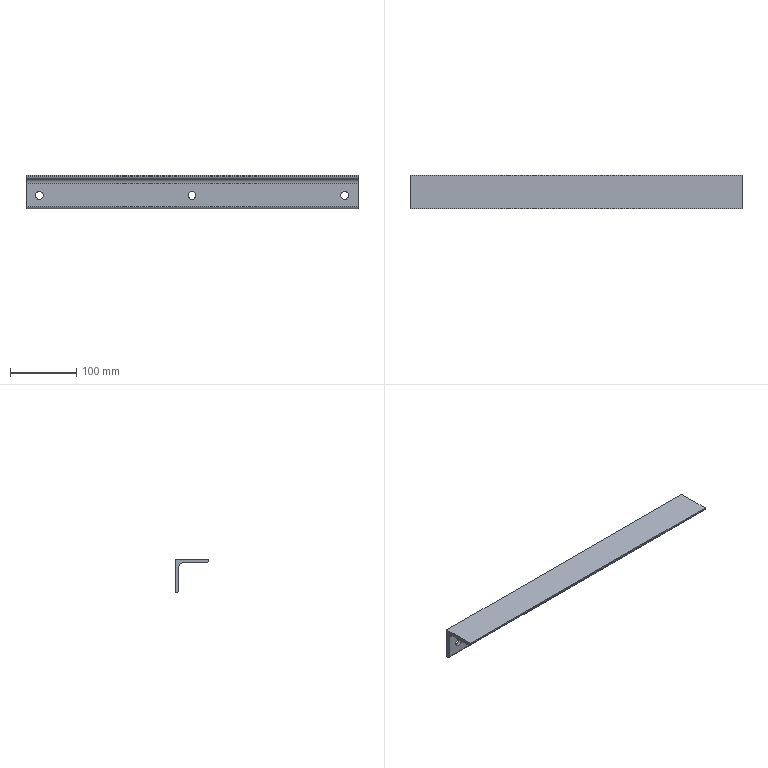Part | STEP file | Input 114 | 1 solid | 17 faces | box 500 x 50 x 50 mm | volume 238406 mm3 | cylinder 9 | plane 8 | commonest cylinder face diameters 12 x6 6 x2 13 x1
STEP:
#1=CARTESIAN_POINT('',(0.,0.,0.));
#2=DIRECTION('',(0.,0.,1.));
#3=DIRECTION('',(1.,0.,0.));
#4=AXIS2_PLACEMENT_3D('',#1,#2,#3);
#5=CARTESIAN_POINT('',(2524.,319.5,-230.));
#6=VERTEX_POINT('',#5);
#7=CARTESIAN_POINT('',(2524.,324.5,-230.));
#8=VERTEX_POINT('',#7);
#9=CARTESIAN_POINT('',(2524.,239.499,-230.));
#10=DIRECTION('',(0.,1.,0.));
#11=VECTOR('',#10,1.);
#12=LINE('',#9,#11);
#13=CARTESIAN_POINT('',(2530.,239.499,-230.));
#14=DIRECTION('',(0.,1.,0.));
#15=DIRECTION('',(-1.,0.,0.));
#16=AXIS2_PLACEMENT_3D('',#13,#14,#15);
#17=CYLINDRICAL_SURFACE('',#16,6.);
#18=CARTESIAN_POINT('',(6.283,0.));
#19=DIRECTION('',(0.,1.));
#20=VECTOR('',#19,1.);
#21=LINE('',#18,#20);
#22=(GEOMETRIC_REPRESENTATION_CONTEXT(2)PARAMETRIC_REPRESENTATION_CONTEXT()REPRESENTATION_CONTEXT('',''));
#23=DEFINITIONAL_REPRESENTATION('',(#21),#22);
#24=PCURVE('',#17,#23);
#25=CARTESIAN_POINT('',(2530.,239.499,-230.));
#26=DIRECTION('',(0.,1.,0.));
#27=DIRECTION('',(-1.,0.,0.));
#28=AXIS2_PLACEMENT_3D('',#25,#26,#27);
#29=CYLINDRICAL_SURFACE('',#28,6.);
#30=CARTESIAN_POINT('',(0.,0.));
#31=DIRECTION('',(0.,1.));
#32=VECTOR('',#31,1.);
#33=LINE('',#30,#32);
#34=(GEOMETRIC_REPRESENTATION_CONTEXT(2)PARAMETRIC_REPRESENTATION_CONTEXT()REPRESENTATION_CONTEXT('',''));
#35=DEFINITIONAL_REPRESENTATION('',(#33),#34);
#36=PCURVE('',#29,#35);
#37=SURFACE_CURVE('',#12,(#24,#36),.PCURVE_S1.);
#38=EDGE_CURVE('',#6,#8,#37,.T.);
#39=ORIENTED_EDGE('',*,*,#38,.T.);
#40=CARTESIAN_POINT('',(2536.,324.5,-230.));
#41=VERTEX_POINT('',#40);
#42=CARTESIAN_POINT('',(2530.,324.5,-230.));
#43=DIRECTION('',(0.,1.,0.));
#44=DIRECTION('',(-1.,0.,0.));
#45=AXIS2_PLACEMENT_3D('',#42,#43,#44);
#46=CIRCLE('',#45,6.);
#47=CARTESIAN_POINT('',(0.,85.001));
#48=DIRECTION('',(1.,0.));
#49=VECTOR('',#48,1.);
#50=LINE('',#47,#49);
#51=(GEOMETRIC_REPRESENTATION_CONTEXT(2)PARAMETRIC_REPRESENTATION_CONTEXT()REPRESENTATION_CONTEXT('',''));
#52=DEFINITIONAL_REPRESENTATION('',(#50),#51);
#53=PCURVE('',#17,#52);
#54=CARTESIAN_POINT('',(2510.,324.5,-200.));
#55=DIRECTION('',(0.,1.,0.));
#56=DIRECTION('',(-1.,0.,0.));
#57=AXIS2_PLACEMENT_3D('',#54,#55,#56);
#58=PLANE('',#57);
#59=CARTESIAN_POINT('',(-20.,-30.));
#60=DIRECTION('',(1.,0.));
#61=AXIS2_PLACEMENT_2D('',#59,#60);
#62=CIRCLE('',#61,6.);
#63=(GEOMETRIC_REPRESENTATION_CONTEXT(2)PARAMETRIC_REPRESENTATION_CONTEXT()REPRESENTATION_CONTEXT('',''));
#64=DEFINITIONAL_REPRESENTATION('',(#62),#63);
#65=PCURVE('',#58,#64);
#66=SURFACE_CURVE('',#46,(#53,#65),.PCURVE_S1.);
#67=EDGE_CURVE('',#41,#8,#66,.T.);
#68=ORIENTED_EDGE('',*,*,#67,.F.);
#69=CARTESIAN_POINT('',(2536.,319.5,-230.));
#70=VERTEX_POINT('',#69);
#71=CARTESIAN_POINT('',(2536.,239.499,-230.));
#72=DIRECTION('',(0.,1.,0.));
#73=VECTOR('',#72,1.);
#74=LINE('',#71,#73);
#75=CARTESIAN_POINT('',(3.142,0.));
#76=DIRECTION('',(0.,1.));
#77=VECTOR('',#76,1.);
#78=LINE('',#75,#77);
#79=(GEOMETRIC_REPRESENTATION_CONTEXT(2)PARAMETRIC_REPRESENTATION_CONTEXT()REPRESENTATION_CONTEXT('',''));
#80=DEFINITIONAL_REPRESENTATION('',(#78),#79);
#81=PCURVE('',#17,#80);
#82=CARTESIAN_POINT('',(3.142,0.));
#83=DIRECTION('',(0.,1.));
#84=VECTOR('',#83,1.);
#85=LINE('',#82,#84);
#86=(GEOMETRIC_REPRESENTATION_CONTEXT(2)PARAMETRIC_REPRESENTATION_CONTEXT()REPRESENTATION_CONTEXT('',''));
#87=DEFINITIONAL_REPRESENTATION('',(#85),#86);
#88=PCURVE('',#29,#87);
#89=SURFACE_CURVE('',#74,(#81,#88),.PCURVE_S1.);
#90=EDGE_CURVE('',#70,#41,#89,.T.);
#91=ORIENTED_EDGE('',*,*,#90,.F.);
#92=CARTESIAN_POINT('',(2530.,319.5,-230.));
#93=DIRECTION('',(0.,1.,0.));
#94=DIRECTION('',(0.,0.,1.));
#95=AXIS2_PLACEMENT_3D('',#92,#93,#94);
#96=CIRCLE('',#95,6.);
#97=CARTESIAN_POINT('',(1.571,80.001));
#98=DIRECTION('',(1.,0.));
#99=VECTOR('',#98,1.);
#100=LINE('',#97,#99);
#101=(GEOMETRIC_REPRESENTATION_CONTEXT(2)PARAMETRIC_REPRESENTATION_CONTEXT()REPRESENTATION_CONTEXT('',''));
#102=DEFINITIONAL_REPRESENTATION('',(#100),#101);
#103=PCURVE('',#17,#102);
#104=CARTESIAN_POINT('',(2510.,319.5,-247.));
#105=DIRECTION('',(0.,-1.,0.));
#106=DIRECTION('',(0.,0.,1.));
#107=AXIS2_PLACEMENT_3D('',#104,#105,#106);
#108=PLANE('',#107);
#109=CARTESIAN_POINT('',(23.,-20.));
#110=CARTESIAN_POINT('',(23.,-30.392));
#111=CARTESIAN_POINT('',(14.,-25.196));
#112=CARTESIAN_POINT('',(5.,-20.));
#113=CARTESIAN_POINT('',(14.,-14.804));
#114=CARTESIAN_POINT('',(23.,-9.608));
#115=CARTESIAN_POINT('',(23.,-20.));
#116=(BOUNDED_CURVE()B_SPLINE_CURVE(2,(#109,#110,#111,#112,#113,#114,#115),.UNSPECIFIED.,.T.,.F.)B_SPLINE_CURVE_WITH_KNOTS((1,2,2,2,2,1),(-2.094,0.,2.094,4.189,6.283,8.378),.UNSPECIFIED.)CURVE()GEOMETRIC_REPRESENTATION_ITEM()RATIONAL_B_SPLINE_CURVE((1.,0.5,1.,0.5,1.,0.5,1.))REPRESENTATION_ITEM(''));
#117=(GEOMETRIC_REPRESENTATION_CONTEXT(2)PARAMETRIC_REPRESENTATION_CONTEXT()REPRESENTATION_CONTEXT('',''));
#118=DEFINITIONAL_REPRESENTATION('',(#116),#117);
#119=PCURVE('',#108,#118);
#120=SURFACE_CURVE('',#96,(#103,#119),.PCURVE_S1.);
#121=EDGE_CURVE('',#70,#6,#120,.T.);
#122=ORIENTED_EDGE('',*,*,#121,.T.);
#123=EDGE_LOOP('',(#39,#68,#91,#122));
#124=FACE_BOUND('',#123,.F.);
#125=ADVANCED_FACE('',(#124),#17,.F.);
#126=CARTESIAN_POINT('',(2754.,319.5,-230.));
#127=VERTEX_POINT('',#126);
#128=CARTESIAN_POINT('',(2754.,324.5,-230.));
#129=VERTEX_POINT('',#128);
#130=CARTESIAN_POINT('',(2754.,239.499,-230.));
#131=DIRECTION('',(0.,1.,0.));
#132=VECTOR('',#131,1.);
#133=LINE('',#130,#132);
#134=CARTESIAN_POINT('',(2760.,239.499,-230.));
#135=DIRECTION('',(0.,1.,0.));
#136=DIRECTION('',(-1.,0.,0.));
#137=AXIS2_PLACEMENT_3D('',#134,#135,#136);
#138=CYLINDRICAL_SURFACE('',#137,6.);
#139=CARTESIAN_POINT('',(6.283,0.));
#140=DIRECTION('',(0.,1.));
#141=VECTOR('',#140,1.);
#142=LINE('',#139,#141);
#143=(GEOMETRIC_REPRESENTATION_CONTEXT(2)PARAMETRIC_REPRESENTATION_CONTEXT()REPRESENTATION_CONTEXT('',''));
#144=DEFINITIONAL_REPRESENTATION('',(#142),#143);
#145=PCURVE('',#138,#144);
#146=CARTESIAN_POINT('',(2760.,239.499,-230.));
#147=DIRECTION('',(0.,1.,0.));
#148=DIRECTION('',(-1.,0.,0.));
#149=AXIS2_PLACEMENT_3D('',#146,#147,#148);
#150=CYLINDRICAL_SURFACE('',#149,6.);
#151=CARTESIAN_POINT('',(0.,0.));
#152=DIRECTION('',(0.,1.));
#153=VECTOR('',#152,1.);
#154=LINE('',#151,#153);
#155=(GEOMETRIC_REPRESENTATION_CONTEXT(2)PARAMETRIC_REPRESENTATION_CONTEXT()REPRESENTATION_CONTEXT('',''));
#156=DEFINITIONAL_REPRESENTATION('',(#154),#155);
#157=PCURVE('',#150,#156);
#158=SURFACE_CURVE('',#133,(#145,#157),.PCURVE_S1.);
#159=EDGE_CURVE('',#127,#129,#158,.T.);
#160=ORIENTED_EDGE('',*,*,#159,.T.);
#161=CARTESIAN_POINT('',(2766.,324.5,-230.));
#162=VERTEX_POINT('',#161);
#163=CARTESIAN_POINT('',(2760.,324.5,-230.));
#164=DIRECTION('',(0.,1.,0.));
#165=DIRECTION('',(-1.,0.,0.));
#166=AXIS2_PLACEMENT_3D('',#163,#164,#165);
#167=CIRCLE('',#166,6.);
#168=CARTESIAN_POINT('',(0.,85.001));
#169=DIRECTION('',(1.,0.));
#170=VECTOR('',#169,1.);
#171=LINE('',#168,#170);
#172=(GEOMETRIC_REPRESENTATION_CONTEXT(2)PARAMETRIC_REPRESENTATION_CONTEXT()REPRESENTATION_CONTEXT('',''));
#173=DEFINITIONAL_REPRESENTATION('',(#171),#172);
#174=PCURVE('',#138,#173);
#175=CARTESIAN_POINT('',(-250.,-30.));
#176=DIRECTION('',(1.,0.));
#177=AXIS2_PLACEMENT_2D('',#175,#176);
#178=CIRCLE('',#177,6.);
#179=(GEOMETRIC_REPRESENTATION_CONTEXT(2)PARAMETRIC_REPRESENTATION_CONTEXT()REPRESENTATION_CONTEXT('',''));
#180=DEFINITIONAL_REPRESENTATION('',(#178),#179);
#181=PCURVE('',#58,#180);
#182=SURFACE_CURVE('',#167,(#174,#181),.PCURVE_S1.);
#183=EDGE_CURVE('',#162,#129,#182,.T.);
#184=ORIENTED_EDGE('',*,*,#183,.F.);
#185=CARTESIAN_POINT('',(2766.,319.5,-230.));
#186=VERTEX_POINT('',#185);
#187=CARTESIAN_POINT('',(2766.,239.499,-230.));
#188=DIRECTION('',(0.,1.,0.));
#189=VECTOR('',#188,1.);
#190=LINE('',#187,#189);
#191=CARTESIAN_POINT('',(3.142,0.));
#192=DIRECTION('',(0.,1.));
#193=VECTOR('',#192,1.);
#194=LINE('',#191,#193);
#195=(GEOMETRIC_REPRESENTATION_CONTEXT(2)PARAMETRIC_REPRESENTATION_CONTEXT()REPRESENTATION_CONTEXT('',''));
#196=DEFINITIONAL_REPRESENTATION('',(#194),#195);
#197=PCURVE('',#138,#196);
#198=CARTESIAN_POINT('',(3.142,0.));
#199=DIRECTION('',(0.,1.));
#200=VECTOR('',#199,1.);
#201=LINE('',#198,#200);
#202=(GEOMETRIC_REPRESENTATION_CONTEXT(2)PARAMETRIC_REPRESENTATION_CONTEXT()REPRESENTATION_CONTEXT('',''));
#203=DEFINITIONAL_REPRESENTATION('',(#201),#202);
#204=PCURVE('',#150,#203);
#205=SURFACE_CURVE('',#190,(#197,#204),.PCURVE_S1.);
#206=EDGE_CURVE('',#186,#162,#205,.T.);
#207=ORIENTED_EDGE('',*,*,#206,.F.);
#208=CARTESIAN_POINT('',(2760.,319.5,-230.));
#209=DIRECTION('',(0.,1.,0.));
#210=DIRECTION('',(0.,0.,1.));
#211=AXIS2_PLACEMENT_3D('',#208,#209,#210);
#212=CIRCLE('',#211,6.);
#213=CARTESIAN_POINT('',(1.571,80.001));
#214=DIRECTION('',(1.,0.));
#215=VECTOR('',#214,1.);
#216=LINE('',#213,#215);
#217=(GEOMETRIC_REPRESENTATION_CONTEXT(2)PARAMETRIC_REPRESENTATION_CONTEXT()REPRESENTATION_CONTEXT('',''));
#218=DEFINITIONAL_REPRESENTATION('',(#216),#217);
#219=PCURVE('',#138,#218);
#220=CARTESIAN_POINT('',(23.,-250.));
#221=CARTESIAN_POINT('',(23.,-260.392));
#222=CARTESIAN_POINT('',(14.,-255.196));
#223=CARTESIAN_POINT('',(5.,-250.));
#224=CARTESIAN_POINT('',(14.,-244.804));
#225=CARTESIAN_POINT('',(23.,-239.608));
#226=CARTESIAN_POINT('',(23.,-250.));
#227=(BOUNDED_CURVE()B_SPLINE_CURVE(2,(#220,#221,#222,#223,#224,#225,#226),.UNSPECIFIED.,.T.,.F.)B_SPLINE_CURVE_WITH_KNOTS((1,2,2,2,2,1),(-2.094,0.,2.094,4.189,6.283,8.378),.UNSPECIFIED.)CURVE()GEOMETRIC_REPRESENTATION_ITEM()RATIONAL_B_SPLINE_CURVE((1.,0.5,1.,0.5,1.,0.5,1.))REPRESENTATION_ITEM(''));
#228=(GEOMETRIC_REPRESENTATION_CONTEXT(2)PARAMETRIC_REPRESENTATION_CONTEXT()REPRESENTATION_CONTEXT('',''));
#229=DEFINITIONAL_REPRESENTATION('',(#227),#228);
#230=PCURVE('',#108,#229);
#231=SURFACE_CURVE('',#212,(#219,#230),.PCURVE_S1.);
#232=EDGE_CURVE('',#186,#127,#231,.T.);
#233=ORIENTED_EDGE('',*,*,#232,.T.);
#234=EDGE_LOOP('',(#160,#184,#207,#233));
#235=FACE_BOUND('',#234,.F.);
#236=ADVANCED_FACE('',(#235),#138,.F.);
#237=CARTESIAN_POINT('',(2984.,319.5,-230.));
#238=VERTEX_POINT('',#237);
#239=CARTESIAN_POINT('',(2984.,324.5,-230.));
#240=VERTEX_POINT('',#239);
#241=CARTESIAN_POINT('',(2984.,239.499,-230.));
#242=DIRECTION('',(0.,1.,0.));
#243=VECTOR('',#242,1.);
#244=LINE('',#241,#243);
#245=CARTESIAN_POINT('',(2990.,239.499,-230.));
#246=DIRECTION('',(0.,1.,0.));
#247=DIRECTION('',(-1.,0.,0.));
#248=AXIS2_PLACEMENT_3D('',#245,#246,#247);
#249=CYLINDRICAL_SURFACE('',#248,6.);
#250=CARTESIAN_POINT('',(6.283,0.));
#251=DIRECTION('',(0.,1.));
#252=VECTOR('',#251,1.);
#253=LINE('',#250,#252);
#254=(GEOMETRIC_REPRESENTATION_CONTEXT(2)PARAMETRIC_REPRESENTATION_CONTEXT()REPRESENTATION_CONTEXT('',''));
#255=DEFINITIONAL_REPRESENTATION('',(#253),#254);
#256=PCURVE('',#249,#255);
#257=CARTESIAN_POINT('',(2990.,239.499,-230.));
#258=DIRECTION('',(0.,1.,0.));
#259=DIRECTION('',(-1.,0.,0.));
#260=AXIS2_PLACEMENT_3D('',#257,#258,#259);
#261=CYLINDRICAL_SURFACE('',#260,6.);
#262=CARTESIAN_POINT('',(0.,0.));
#263=DIRECTION('',(0.,1.));
#264=VECTOR('',#263,1.);
#265=LINE('',#262,#264);
#266=(GEOMETRIC_REPRESENTATION_CONTEXT(2)PARAMETRIC_REPRESENTATION_CONTEXT()REPRESENTATION_CONTEXT('',''));
#267=DEFINITIONAL_REPRESENTATION('',(#265),#266);
#268=PCURVE('',#261,#267);
#269=SURFACE_CURVE('',#244,(#256,#268),.PCURVE_S1.);
#270=EDGE_CURVE('',#238,#240,#269,.T.);
#271=ORIENTED_EDGE('',*,*,#270,.T.);
#272=CARTESIAN_POINT('',(2996.,324.5,-230.));
#273=VERTEX_POINT('',#272);
#274=CARTESIAN_POINT('',(2990.,324.5,-230.));
#275=DIRECTION('',(0.,1.,0.));
#276=DIRECTION('',(-1.,0.,0.));
#277=AXIS2_PLACEMENT_3D('',#274,#275,#276);
#278=CIRCLE('',#277,6.);
#279=CARTESIAN_POINT('',(0.,85.001));
#280=DIRECTION('',(1.,0.));
#281=VECTOR('',#280,1.);
#282=LINE('',#279,#281);
#283=(GEOMETRIC_REPRESENTATION_CONTEXT(2)PARAMETRIC_REPRESENTATION_CONTEXT()REPRESENTATION_CONTEXT('',''));
#284=DEFINITIONAL_REPRESENTATION('',(#282),#283);
#285=PCURVE('',#249,#284);
#286=CARTESIAN_POINT('',(-480.,-30.));
#287=DIRECTION('',(1.,0.));
#288=AXIS2_PLACEMENT_2D('',#286,#287);
#289=CIRCLE('',#288,6.);
#290=(GEOMETRIC_REPRESENTATION_CONTEXT(2)PARAMETRIC_REPRESENTATION_CONTEXT()REPRESENTATION_CONTEXT('',''));
#291=DEFINITIONAL_REPRESENTATION('',(#289),#290);
#292=PCURVE('',#58,#291);
#293=SURFACE_CURVE('',#278,(#285,#292),.PCURVE_S1.);
#294=EDGE_CURVE('',#273,#240,#293,.T.);
#295=ORIENTED_EDGE('',*,*,#294,.F.);
#296=CARTESIAN_POINT('',(2996.,319.5,-230.));
#297=VERTEX_POINT('',#296);
#298=CARTESIAN_POINT('',(2996.,239.499,-230.));
#299=DIRECTION('',(0.,1.,0.));
#300=VECTOR('',#299,1.);
#301=LINE('',#298,#300);
#302=CARTESIAN_POINT('',(3.142,0.));
#303=DIRECTION('',(0.,1.));
#304=VECTOR('',#303,1.);
#305=LINE('',#302,#304);
#306=(GEOMETRIC_REPRESENTATION_CONTEXT(2)PARAMETRIC_REPRESENTATION_CONTEXT()REPRESENTATION_CONTEXT('',''));
#307=DEFINITIONAL_REPRESENTATION('',(#305),#306);
#308=PCURVE('',#249,#307);
#309=CARTESIAN_POINT('',(3.142,0.));
#310=DIRECTION('',(0.,1.));
#311=VECTOR('',#310,1.);
#312=LINE('',#309,#311);
#313=(GEOMETRIC_REPRESENTATION_CONTEXT(2)PARAMETRIC_REPRESENTATION_CONTEXT()REPRESENTATION_CONTEXT('',''));
#314=DEFINITIONAL_REPRESENTATION('',(#312),#313);
#315=PCURVE('',#261,#314);
#316=SURFACE_CURVE('',#301,(#308,#315),.PCURVE_S1.);
#317=EDGE_CURVE('',#297,#273,#316,.T.);
#318=ORIENTED_EDGE('',*,*,#317,.F.);
#319=CARTESIAN_POINT('',(2990.,319.5,-230.));
#320=DIRECTION('',(0.,1.,0.));
#321=DIRECTION('',(0.,0.,1.));
#322=AXIS2_PLACEMENT_3D('',#319,#320,#321);
#323=CIRCLE('',#322,6.);
#324=CARTESIAN_POINT('',(1.571,80.001));
#325=DIRECTION('',(1.,0.));
#326=VECTOR('',#325,1.);
#327=LINE('',#324,#326);
#328=(GEOMETRIC_REPRESENTATION_CONTEXT(2)PARAMETRIC_REPRESENTATION_CONTEXT()REPRESENTATION_CONTEXT('',''));
#329=DEFINITIONAL_REPRESENTATION('',(#327),#328);
#330=PCURVE('',#249,#329);
#331=CARTESIAN_POINT('',(23.,-480.));
#332=CARTESIAN_POINT('',(23.,-490.392));
#333=CARTESIAN_POINT('',(14.,-485.196));
#334=CARTESIAN_POINT('',(5.,-480.));
#335=CARTESIAN_POINT('',(14.,-474.804));
#336=CARTESIAN_POINT('',(23.,-469.608));
#337=CARTESIAN_POINT('',(23.,-480.));
#338=(BOUNDED_CURVE()B_SPLINE_CURVE(2,(#331,#332,#333,#334,#335,#336,#337),.UNSPECIFIED.,.T.,.F.)B_SPLINE_CURVE_WITH_KNOTS((1,2,2,2,2,1),(-2.094,0.,2.094,4.189,6.283,8.378),.UNSPECIFIED.)CURVE()GEOMETRIC_REPRESENTATION_ITEM()RATIONAL_B_SPLINE_CURVE((1.,0.5,1.,0.5,1.,0.5,1.))REPRESENTATION_ITEM(''));
#339=(GEOMETRIC_REPRESENTATION_CONTEXT(2)PARAMETRIC_REPRESENTATION_CONTEXT()REPRESENTATION_CONTEXT('',''));
#340=DEFINITIONAL_REPRESENTATION('',(#338),#339);
#341=PCURVE('',#108,#340);
#342=SURFACE_CURVE('',#323,(#330,#341),.PCURVE_S1.);
#343=EDGE_CURVE('',#297,#238,#342,.T.);
#344=ORIENTED_EDGE('',*,*,#343,.T.);
#345=EDGE_LOOP('',(#271,#295,#318,#344));
#346=FACE_BOUND('',#345,.F.);
#347=ADVANCED_FACE('',(#346),#249,.F.);
#348=CARTESIAN_POINT('',(3010.,324.5,-200.));
#349=VERTEX_POINT('',#348);
#350=CARTESIAN_POINT('',(3010.,274.5,-200.));
#351=VERTEX_POINT('',#350);
#352=CARTESIAN_POINT('',(3010.,274.5,-200.));
#353=DIRECTION('',(0.,-1.,0.));
#354=VECTOR('',#353,1.);
#355=LINE('',#352,#354);
#356=CARTESIAN_POINT('',(2510.,274.5,-200.));
#357=DIRECTION('',(0.,0.,1.));
#358=DIRECTION('',(1.,0.,0.));
#359=AXIS2_PLACEMENT_3D('',#356,#357,#358);
#360=PLANE('',#359);
#361=CARTESIAN_POINT('',(500.,0.));
#362=DIRECTION('',(0.,-1.));
#363=VECTOR('',#362,1.);
#364=LINE('',#361,#363);
#365=(GEOMETRIC_REPRESENTATION_CONTEXT(2)PARAMETRIC_REPRESENTATION_CONTEXT()REPRESENTATION_CONTEXT('',''));
#366=DEFINITIONAL_REPRESENTATION('',(#364),#365);
#367=PCURVE('',#360,#366);
#368=CARTESIAN_POINT('',(3010.,322.5,-247.));
#369=DIRECTION('',(-1.,0.,0.));
#370=DIRECTION('',(0.,0.,1.));
#371=AXIS2_PLACEMENT_3D('',#368,#369,#370);
#372=PLANE('',#371);
#373=CARTESIAN_POINT('',(47.,-48.));
#374=DIRECTION('',(0.,-1.));
#375=VECTOR('',#374,1.);
#376=LINE('',#373,#375);
#377=(GEOMETRIC_REPRESENTATION_CONTEXT(2)PARAMETRIC_REPRESENTATION_CONTEXT()REPRESENTATION_CONTEXT('',''));
#378=DEFINITIONAL_REPRESENTATION('',(#376),#377);
#379=PCURVE('',#372,#378);
#380=SURFACE_CURVE('',#355,(#367,#379),.PCURVE_S1.);
#381=EDGE_CURVE('',#349,#351,#380,.T.);
#382=ORIENTED_EDGE('',*,*,#381,.F.);
#383=CARTESIAN_POINT('',(2510.,324.5,-200.));
#384=VERTEX_POINT('',#383);
#385=CARTESIAN_POINT('',(2510.,324.5,-200.));
#386=DIRECTION('',(1.,0.,0.));
#387=VECTOR('',#386,1.);
#388=LINE('',#385,#387);
#389=CARTESIAN_POINT('',(0.,50.));
#390=DIRECTION('',(1.,0.));
#391=VECTOR('',#390,1.);
#392=LINE('',#389,#391);
#393=(GEOMETRIC_REPRESENTATION_CONTEXT(2)PARAMETRIC_REPRESENTATION_CONTEXT()REPRESENTATION_CONTEXT('',''));
#394=DEFINITIONAL_REPRESENTATION('',(#392),#393);
#395=PCURVE('',#360,#394);
#396=CARTESIAN_POINT('',(0.,0.));
#397=DIRECTION('',(-1.,0.));
#398=VECTOR('',#397,1.);
#399=LINE('',#396,#398);
#400=(GEOMETRIC_REPRESENTATION_CONTEXT(2)PARAMETRIC_REPRESENTATION_CONTEXT()REPRESENTATION_CONTEXT('',''));
#401=DEFINITIONAL_REPRESENTATION('',(#399),#400);
#402=PCURVE('',#58,#401);
#403=SURFACE_CURVE('',#388,(#395,#402),.PCURVE_S1.);
#404=EDGE_CURVE('',#384,#349,#403,.T.);
#405=ORIENTED_EDGE('',*,*,#404,.F.);
#406=CARTESIAN_POINT('',(2510.,274.5,-200.));
#407=VERTEX_POINT('',#406);
#408=CARTESIAN_POINT('',(2510.,274.5,-200.));
#409=DIRECTION('',(0.,-1.,0.));
#410=VECTOR('',#409,1.);
#411=LINE('',#408,#410);
#412=CARTESIAN_POINT('',(0.,0.));
#413=DIRECTION('',(0.,-1.));
#414=VECTOR('',#413,1.);
#415=LINE('',#412,#414);
#416=(GEOMETRIC_REPRESENTATION_CONTEXT(2)PARAMETRIC_REPRESENTATION_CONTEXT()REPRESENTATION_CONTEXT('',''));
#417=DEFINITIONAL_REPRESENTATION('',(#415),#416);
#418=PCURVE('',#360,#417);
#419=CARTESIAN_POINT('',(2510.,322.5,-247.));
#420=DIRECTION('',(-1.,0.,0.));
#421=DIRECTION('',(0.,0.,1.));
#422=AXIS2_PLACEMENT_3D('',#419,#420,#421);
#423=PLANE('',#422);
#424=CARTESIAN_POINT('',(47.,-48.));
#425=DIRECTION('',(0.,-1.));
#426=VECTOR('',#425,1.);
#427=LINE('',#424,#426);
#428=(GEOMETRIC_REPRESENTATION_CONTEXT(2)PARAMETRIC_REPRESENTATION_CONTEXT()REPRESENTATION_CONTEXT('',''));
#429=DEFINITIONAL_REPRESENTATION('',(#427),#428);
#430=PCURVE('',#423,#429);
#431=SURFACE_CURVE('',#411,(#418,#430),.PCURVE_S1.);
#432=EDGE_CURVE('',#384,#407,#431,.T.);
#433=ORIENTED_EDGE('',*,*,#432,.T.);
#434=CARTESIAN_POINT('',(2510.,274.5,-200.));
#435=DIRECTION('',(1.,0.,0.));
#436=VECTOR('',#435,1.);
#437=LINE('',#434,#436);
#438=CARTESIAN_POINT('',(0.,0.));
#439=DIRECTION('',(1.,0.));
#440=VECTOR('',#439,1.);
#441=LINE('',#438,#440);
#442=(GEOMETRIC_REPRESENTATION_CONTEXT(2)PARAMETRIC_REPRESENTATION_CONTEXT()REPRESENTATION_CONTEXT('',''));
#443=DEFINITIONAL_REPRESENTATION('',(#441),#442);
#444=PCURVE('',#360,#443);
#445=CARTESIAN_POINT('',(2510.,274.5,-200.));
#446=DIRECTION('',(0.,-1.,0.));
#447=DIRECTION('',(1.,0.,0.));
#448=AXIS2_PLACEMENT_3D('',#445,#446,#447);
#449=PLANE('',#448);
#450=CARTESIAN_POINT('',(0.,0.));
#451=DIRECTION('',(1.,0.));
#452=VECTOR('',#451,1.);
#453=LINE('',#450,#452);
#454=(GEOMETRIC_REPRESENTATION_CONTEXT(2)PARAMETRIC_REPRESENTATION_CONTEXT()REPRESENTATION_CONTEXT('',''));
#455=DEFINITIONAL_REPRESENTATION('',(#453),#454);
#456=PCURVE('',#449,#455);
#457=SURFACE_CURVE('',#437,(#444,#456),.PCURVE_S1.);
#458=EDGE_CURVE('',#407,#351,#457,.T.);
#459=ORIENTED_EDGE('',*,*,#458,.T.);
#460=EDGE_LOOP('',(#382,#405,#433,#459));
#461=FACE_BOUND('',#460,.T.);
#462=ADVANCED_FACE('',(#461),#360,.T.);
#463=CARTESIAN_POINT('',(2530.,324.5,-230.));
#464=DIRECTION('',(0.,1.,0.));
#465=DIRECTION('',(-1.,0.,0.));
#466=AXIS2_PLACEMENT_3D('',#463,#464,#465);
#467=CIRCLE('',#466,6.);
#468=CARTESIAN_POINT('',(-20.,-30.));
#469=DIRECTION('',(1.,0.));
#470=AXIS2_PLACEMENT_2D('',#468,#469);
#471=CIRCLE('',#470,6.);
#472=(GEOMETRIC_REPRESENTATION_CONTEXT(2)PARAMETRIC_REPRESENTATION_CONTEXT()REPRESENTATION_CONTEXT('',''));
#473=DEFINITIONAL_REPRESENTATION('',(#471),#472);
#474=PCURVE('',#58,#473);
#475=CARTESIAN_POINT('',(0.,85.001));
#476=DIRECTION('',(1.,0.));
#477=VECTOR('',#476,1.);
#478=LINE('',#475,#477);
#479=(GEOMETRIC_REPRESENTATION_CONTEXT(2)PARAMETRIC_REPRESENTATION_CONTEXT()REPRESENTATION_CONTEXT('',''));
#480=DEFINITIONAL_REPRESENTATION('',(#478),#479);
#481=PCURVE('',#29,#480);
#482=SURFACE_CURVE('',#467,(#474,#481),.PCURVE_S1.);
#483=EDGE_CURVE('',#8,#41,#482,.T.);
#484=ORIENTED_EDGE('',*,*,#483,.F.);
#485=ORIENTED_EDGE('',*,*,#67,.F.);
#486=EDGE_LOOP('',(#484,#485));
#487=FACE_BOUND('',#486,.T.);
#488=CARTESIAN_POINT('',(2760.,324.5,-230.));
#489=DIRECTION('',(0.,1.,0.));
#490=DIRECTION('',(-1.,0.,0.));
#491=AXIS2_PLACEMENT_3D('',#488,#489,#490);
#492=CIRCLE('',#491,6.);
#493=CARTESIAN_POINT('',(-250.,-30.));
#494=DIRECTION('',(1.,0.));
#495=AXIS2_PLACEMENT_2D('',#493,#494);
#496=CIRCLE('',#495,6.);
#497=(GEOMETRIC_REPRESENTATION_CONTEXT(2)PARAMETRIC_REPRESENTATION_CONTEXT()REPRESENTATION_CONTEXT('',''));
#498=DEFINITIONAL_REPRESENTATION('',(#496),#497);
#499=PCURVE('',#58,#498);
#500=CARTESIAN_POINT('',(0.,85.001));
#501=DIRECTION('',(1.,0.));
#502=VECTOR('',#501,1.);
#503=LINE('',#500,#502);
#504=(GEOMETRIC_REPRESENTATION_CONTEXT(2)PARAMETRIC_REPRESENTATION_CONTEXT()REPRESENTATION_CONTEXT('',''));
#505=DEFINITIONAL_REPRESENTATION('',(#503),#504);
#506=PCURVE('',#150,#505);
#507=SURFACE_CURVE('',#492,(#499,#506),.PCURVE_S1.);
#508=EDGE_CURVE('',#129,#162,#507,.T.);
#509=ORIENTED_EDGE('',*,*,#508,.F.);
#510=ORIENTED_EDGE('',*,*,#183,.F.);
#511=EDGE_LOOP('',(#509,#510));
#512=FACE_BOUND('',#511,.T.);
#513=CARTESIAN_POINT('',(2990.,324.5,-230.));
#514=DIRECTION('',(0.,1.,0.));
#515=DIRECTION('',(-1.,0.,0.));
#516=AXIS2_PLACEMENT_3D('',#513,#514,#515);
#517=CIRCLE('',#516,6.);
#518=CARTESIAN_POINT('',(-480.,-30.));
#519=DIRECTION('',(1.,0.));
#520=AXIS2_PLACEMENT_2D('',#518,#519);
#521=CIRCLE('',#520,6.);
#522=(GEOMETRIC_REPRESENTATION_CONTEXT(2)PARAMETRIC_REPRESENTATION_CONTEXT()REPRESENTATION_CONTEXT('',''));
#523=DEFINITIONAL_REPRESENTATION('',(#521),#522);
#524=PCURVE('',#58,#523);
#525=CARTESIAN_POINT('',(0.,85.001));
#526=DIRECTION('',(1.,0.));
#527=VECTOR('',#526,1.);
#528=LINE('',#525,#527);
#529=(GEOMETRIC_REPRESENTATION_CONTEXT(2)PARAMETRIC_REPRESENTATION_CONTEXT()REPRESENTATION_CONTEXT('',''));
#530=DEFINITIONAL_REPRESENTATION('',(#528),#529);
#531=PCURVE('',#261,#530);
#532=SURFACE_CURVE('',#517,(#524,#531),.PCURVE_S1.);
#533=EDGE_CURVE('',#240,#273,#532,.T.);
#534=ORIENTED_EDGE('',*,*,#533,.F.);
#535=ORIENTED_EDGE('',*,*,#294,.F.);
#536=EDGE_LOOP('',(#534,#535));
#537=FACE_BOUND('',#536,.T.);
#538=CARTESIAN_POINT('',(3010.,324.5,-250.));
#539=VERTEX_POINT('',#538);
#540=CARTESIAN_POINT('',(3010.,324.5,-200.));
#541=DIRECTION('',(0.,0.,1.));
#542=VECTOR('',#541,1.);
#543=LINE('',#540,#542);
#544=CARTESIAN_POINT('',(-500.,0.));
#545=DIRECTION('',(0.,1.));
#546=VECTOR('',#545,1.);
#547=LINE('',#544,#546);
#548=(GEOMETRIC_REPRESENTATION_CONTEXT(2)PARAMETRIC_REPRESENTATION_CONTEXT()REPRESENTATION_CONTEXT('',''));
#549=DEFINITIONAL_REPRESENTATION('',(#547),#548);
#550=PCURVE('',#58,#549);
#551=CARTESIAN_POINT('',(47.,2.));
#552=DIRECTION('',(1.,0.));
#553=VECTOR('',#552,1.);
#554=LINE('',#551,#553);
#555=(GEOMETRIC_REPRESENTATION_CONTEXT(2)PARAMETRIC_REPRESENTATION_CONTEXT()REPRESENTATION_CONTEXT('',''));
#556=DEFINITIONAL_REPRESENTATION('',(#554),#555);
#557=PCURVE('',#372,#556);
#558=SURFACE_CURVE('',#543,(#550,#557),.PCURVE_S1.);
#559=EDGE_CURVE('',#539,#349,#558,.T.);
#560=ORIENTED_EDGE('',*,*,#559,.F.);
#561=CARTESIAN_POINT('',(2510.,324.5,-250.));
#562=VERTEX_POINT('',#561);
#563=CARTESIAN_POINT('',(2510.,324.5,-250.));
#564=DIRECTION('',(1.,0.,0.));
#565=VECTOR('',#564,1.);
#566=LINE('',#563,#565);
#567=CARTESIAN_POINT('',(0.,-50.));
#568=DIRECTION('',(-1.,0.));
#569=VECTOR('',#568,1.);
#570=LINE('',#567,#569);
#571=(GEOMETRIC_REPRESENTATION_CONTEXT(2)PARAMETRIC_REPRESENTATION_CONTEXT()REPRESENTATION_CONTEXT('',''));
#572=DEFINITIONAL_REPRESENTATION('',(#570),#571);
#573=PCURVE('',#58,#572);
#574=CARTESIAN_POINT('',(2510.,324.5,-250.));
#575=DIRECTION('',(0.,0.,-1.));
#576=DIRECTION('',(-1.,0.,0.));
#577=AXIS2_PLACEMENT_3D('',#574,#575,#576);
#578=PLANE('',#577);
#579=CARTESIAN_POINT('',(0.,0.));
#580=DIRECTION('',(-1.,0.));
#581=VECTOR('',#580,1.);
#582=LINE('',#579,#581);
#583=(GEOMETRIC_REPRESENTATION_CONTEXT(2)PARAMETRIC_REPRESENTATION_CONTEXT()REPRESENTATION_CONTEXT('',''));
#584=DEFINITIONAL_REPRESENTATION('',(#582),#583);
#585=PCURVE('',#578,#584);
#586=SURFACE_CURVE('',#566,(#573,#585),.PCURVE_S1.);
#587=EDGE_CURVE('',#562,#539,#586,.T.);
#588=ORIENTED_EDGE('',*,*,#587,.F.);
#589=CARTESIAN_POINT('',(2510.,324.5,-200.));
#590=DIRECTION('',(0.,0.,1.));
#591=VECTOR('',#590,1.);
#592=LINE('',#589,#591);
#593=CARTESIAN_POINT('',(0.,0.));
#594=DIRECTION('',(0.,1.));
#595=VECTOR('',#594,1.);
#596=LINE('',#593,#595);
#597=(GEOMETRIC_REPRESENTATION_CONTEXT(2)PARAMETRIC_REPRESENTATION_CONTEXT()REPRESENTATION_CONTEXT('',''));
#598=DEFINITIONAL_REPRESENTATION('',(#596),#597);
#599=PCURVE('',#58,#598);
#600=CARTESIAN_POINT('',(47.,2.));
#601=DIRECTION('',(1.,0.));
#602=VECTOR('',#601,1.);
#603=LINE('',#600,#602);
#604=(GEOMETRIC_REPRESENTATION_CONTEXT(2)PARAMETRIC_REPRESENTATION_CONTEXT()REPRESENTATION_CONTEXT('',''));
#605=DEFINITIONAL_REPRESENTATION('',(#603),#604);
#606=PCURVE('',#423,#605);
#607=SURFACE_CURVE('',#592,(#599,#606),.PCURVE_S1.);
#608=EDGE_CURVE('',#562,#384,#607,.T.);
#609=ORIENTED_EDGE('',*,*,#608,.T.);
#610=ORIENTED_EDGE('',*,*,#404,.T.);
#611=EDGE_LOOP('',(#560,#588,#609,#610));
#612=FACE_BOUND('',#611,.T.);
#613=ADVANCED_FACE('',(#487,#512,#537,#612),#58,.T.);
#614=CARTESIAN_POINT('',(3010.,322.5,-250.));
#615=VERTEX_POINT('',#614);
#616=CARTESIAN_POINT('',(3010.,324.5,-250.));
#617=DIRECTION('',(0.,1.,0.));
#618=VECTOR('',#617,1.);
#619=LINE('',#616,#618);
#620=CARTESIAN_POINT('',(-500.,0.));
#621=DIRECTION('',(0.,1.));
#622=VECTOR('',#621,1.);
#623=LINE('',#620,#622);
#624=(GEOMETRIC_REPRESENTATION_CONTEXT(2)PARAMETRIC_REPRESENTATION_CONTEXT()REPRESENTATION_CONTEXT('',''));
#625=DEFINITIONAL_REPRESENTATION('',(#623),#624);
#626=PCURVE('',#578,#625);
#627=CARTESIAN_POINT('',(-3.,2.));
#628=DIRECTION('',(0.,1.));
#629=VECTOR('',#628,1.);
#630=LINE('',#627,#629);
#631=(GEOMETRIC_REPRESENTATION_CONTEXT(2)PARAMETRIC_REPRESENTATION_CONTEXT()REPRESENTATION_CONTEXT('',''));
#632=DEFINITIONAL_REPRESENTATION('',(#630),#631);
#633=PCURVE('',#372,#632);
#634=SURFACE_CURVE('',#619,(#626,#633),.PCURVE_S1.);
#635=EDGE_CURVE('',#615,#539,#634,.T.);
#636=ORIENTED_EDGE('',*,*,#635,.F.);
#637=CARTESIAN_POINT('',(2510.,322.5,-250.));
#638=VERTEX_POINT('',#637);
#639=CARTESIAN_POINT('',(2510.,322.5,-250.));
#640=DIRECTION('',(1.,0.,0.));
#641=VECTOR('',#640,1.);
#642=LINE('',#639,#641);
#643=CARTESIAN_POINT('',(0.,-2.));
#644=DIRECTION('',(-1.,0.));
#645=VECTOR('',#644,1.);
#646=LINE('',#643,#645);
#647=(GEOMETRIC_REPRESENTATION_CONTEXT(2)PARAMETRIC_REPRESENTATION_CONTEXT()REPRESENTATION_CONTEXT('',''));
#648=DEFINITIONAL_REPRESENTATION('',(#646),#647);
#649=PCURVE('',#578,#648);
#650=CARTESIAN_POINT('',(2510.,322.5,-247.));
#651=DIRECTION('',(1.,0.,0.));
#652=DIRECTION('',(0.,0.,-1.));
#653=AXIS2_PLACEMENT_3D('',#650,#651,#652);
#654=CYLINDRICAL_SURFACE('',#653,3.);
#655=CARTESIAN_POINT('',(6.283,0.));
#656=DIRECTION('',(0.,1.));
#657=VECTOR('',#656,1.);
#658=LINE('',#655,#657);
#659=(GEOMETRIC_REPRESENTATION_CONTEXT(2)PARAMETRIC_REPRESENTATION_CONTEXT()REPRESENTATION_CONTEXT('',''));
#660=DEFINITIONAL_REPRESENTATION('',(#658),#659);
#661=PCURVE('',#654,#660);
#662=SURFACE_CURVE('',#642,(#649,#661),.PCURVE_S1.);
#663=EDGE_CURVE('',#638,#615,#662,.T.);
#664=ORIENTED_EDGE('',*,*,#663,.F.);
#665=CARTESIAN_POINT('',(2510.,324.5,-250.));
#666=DIRECTION('',(0.,1.,0.));
#667=VECTOR('',#666,1.);
#668=LINE('',#665,#667);
#669=CARTESIAN_POINT('',(0.,0.));
#670=DIRECTION('',(0.,1.));
#671=VECTOR('',#670,1.);
#672=LINE('',#669,#671);
#673=(GEOMETRIC_REPRESENTATION_CONTEXT(2)PARAMETRIC_REPRESENTATION_CONTEXT()REPRESENTATION_CONTEXT('',''));
#674=DEFINITIONAL_REPRESENTATION('',(#672),#673);
#675=PCURVE('',#578,#674);
#676=CARTESIAN_POINT('',(-3.,2.));
#677=DIRECTION('',(0.,1.));
#678=VECTOR('',#677,1.);
#679=LINE('',#676,#678);
#680=(GEOMETRIC_REPRESENTATION_CONTEXT(2)PARAMETRIC_REPRESENTATION_CONTEXT()REPRESENTATION_CONTEXT('',''));
#681=DEFINITIONAL_REPRESENTATION('',(#679),#680);
#682=PCURVE('',#423,#681);
#683=SURFACE_CURVE('',#668,(#675,#682),.PCURVE_S1.);
#684=EDGE_CURVE('',#638,#562,#683,.T.);
#685=ORIENTED_EDGE('',*,*,#684,.T.);
#686=ORIENTED_EDGE('',*,*,#587,.T.);
#687=EDGE_LOOP('',(#636,#664,#685,#686));
#688=FACE_BOUND('',#687,.T.);
#689=ADVANCED_FACE('',(#688),#578,.T.);
#690=CARTESIAN_POINT('',(3010.,319.5,-247.));
#691=VERTEX_POINT('',#690);
#692=CARTESIAN_POINT('',(3010.,322.5,-247.));
#693=DIRECTION('',(1.,0.,0.));
#694=DIRECTION('',(0.,0.,1.));
#695=AXIS2_PLACEMENT_3D('',#692,#693,#694);
#696=CIRCLE('',#695,3.);
#697=CARTESIAN_POINT('',(3.142,500.));
#698=DIRECTION('',(1.,0.));
#699=VECTOR('',#698,1.);
#700=LINE('',#697,#699);
#701=(GEOMETRIC_REPRESENTATION_CONTEXT(2)PARAMETRIC_REPRESENTATION_CONTEXT()REPRESENTATION_CONTEXT('',''));
#702=DEFINITIONAL_REPRESENTATION('',(#700),#701);
#703=PCURVE('',#654,#702);
#704=CARTESIAN_POINT('',(3.,0.));
#705=CARTESIAN_POINT('',(3.,-5.196));
#706=CARTESIAN_POINT('',(-1.5,-2.598));
#707=CARTESIAN_POINT('',(-6.,0.));
#708=CARTESIAN_POINT('',(-1.5,2.598));
#709=CARTESIAN_POINT('',(3.,5.196));
#710=CARTESIAN_POINT('',(3.,0.));
#711=(BOUNDED_CURVE()B_SPLINE_CURVE(2,(#704,#705,#706,#707,#708,#709,#710),.UNSPECIFIED.,.T.,.F.)B_SPLINE_CURVE_WITH_KNOTS((1,2,2,2,2,1),(-2.094,0.,2.094,4.189,6.283,8.378),.UNSPECIFIED.)CURVE()GEOMETRIC_REPRESENTATION_ITEM()RATIONAL_B_SPLINE_CURVE((1.,0.5,1.,0.5,1.,0.5,1.))REPRESENTATION_ITEM(''));
#712=(GEOMETRIC_REPRESENTATION_CONTEXT(2)PARAMETRIC_REPRESENTATION_CONTEXT()REPRESENTATION_CONTEXT('',''));
#713=DEFINITIONAL_REPRESENTATION('',(#711),#712);
#714=PCURVE('',#372,#713);
#715=SURFACE_CURVE('',#696,(#703,#714),.PCURVE_S1.);
#716=EDGE_CURVE('',#691,#615,#715,.T.);
#717=ORIENTED_EDGE('',*,*,#716,.F.);
#718=CARTESIAN_POINT('',(2510.,319.5,-247.));
#719=VERTEX_POINT('',#718);
#720=CARTESIAN_POINT('',(2510.,319.5,-247.));
#721=DIRECTION('',(1.,0.,0.));
#722=VECTOR('',#721,1.);
#723=LINE('',#720,#722);
#724=CARTESIAN_POINT('',(4.712,0.));
#725=DIRECTION('',(0.,1.));
#726=VECTOR('',#725,1.);
#727=LINE('',#724,#726);
#728=(GEOMETRIC_REPRESENTATION_CONTEXT(2)PARAMETRIC_REPRESENTATION_CONTEXT()REPRESENTATION_CONTEXT('',''));
#729=DEFINITIONAL_REPRESENTATION('',(#727),#728);
#730=PCURVE('',#654,#729);
#731=CARTESIAN_POINT('',(0.,0.));
#732=DIRECTION('',(0.,-1.));
#733=VECTOR('',#732,1.);
#734=LINE('',#731,#733);
#735=(GEOMETRIC_REPRESENTATION_CONTEXT(2)PARAMETRIC_REPRESENTATION_CONTEXT()REPRESENTATION_CONTEXT('',''));
#736=DEFINITIONAL_REPRESENTATION('',(#734),#735);
#737=PCURVE('',#108,#736);
#738=SURFACE_CURVE('',#723,(#730,#737),.PCURVE_S1.);
#739=EDGE_CURVE('',#719,#691,#738,.T.);
#740=ORIENTED_EDGE('',*,*,#739,.F.);
#741=CARTESIAN_POINT('',(2510.,322.5,-247.));
#742=DIRECTION('',(1.,0.,0.));
#743=DIRECTION('',(0.,0.,1.));
#744=AXIS2_PLACEMENT_3D('',#741,#742,#743);
#745=CIRCLE('',#744,3.);
#746=CARTESIAN_POINT('',(3.142,0.));
#747=DIRECTION('',(1.,0.));
#748=VECTOR('',#747,1.);
#749=LINE('',#746,#748);
#750=(GEOMETRIC_REPRESENTATION_CONTEXT(2)PARAMETRIC_REPRESENTATION_CONTEXT()REPRESENTATION_CONTEXT('',''));
#751=DEFINITIONAL_REPRESENTATION('',(#749),#750);
#752=PCURVE('',#654,#751);
#753=CARTESIAN_POINT('',(3.,0.));
#754=CARTESIAN_POINT('',(3.,-5.196));
#755=CARTESIAN_POINT('',(-1.5,-2.598));
#756=CARTESIAN_POINT('',(-6.,0.));
#757=CARTESIAN_POINT('',(-1.5,2.598));
#758=CARTESIAN_POINT('',(3.,5.196));
#759=CARTESIAN_POINT('',(3.,0.));
#760=(BOUNDED_CURVE()B_SPLINE_CURVE(2,(#753,#754,#755,#756,#757,#758,#759),.UNSPECIFIED.,.T.,.F.)B_SPLINE_CURVE_WITH_KNOTS((1,2,2,2,2,1),(-2.094,0.,2.094,4.189,6.283,8.378),.UNSPECIFIED.)CURVE()GEOMETRIC_REPRESENTATION_ITEM()RATIONAL_B_SPLINE_CURVE((1.,0.5,1.,0.5,1.,0.5,1.))REPRESENTATION_ITEM(''));
#761=(GEOMETRIC_REPRESENTATION_CONTEXT(2)PARAMETRIC_REPRESENTATION_CONTEXT()REPRESENTATION_CONTEXT('',''));
#762=DEFINITIONAL_REPRESENTATION('',(#760),#761);
#763=PCURVE('',#423,#762);
#764=SURFACE_CURVE('',#745,(#752,#763),.PCURVE_S1.);
#765=EDGE_CURVE('',#719,#638,#764,.T.);
#766=ORIENTED_EDGE('',*,*,#765,.T.);
#767=ORIENTED_EDGE('',*,*,#663,.T.);
#768=EDGE_LOOP('',(#717,#740,#766,#767));
#769=FACE_BOUND('',#768,.T.);
#770=ADVANCED_FACE('',(#769),#654,.T.);
#771=CARTESIAN_POINT('',(2530.,319.5,-230.));
#772=DIRECTION('',(0.,1.,0.));
#773=DIRECTION('',(0.,0.,1.));
#774=AXIS2_PLACEMENT_3D('',#771,#772,#773);
#775=CIRCLE('',#774,6.);
#776=CARTESIAN_POINT('',(23.,-20.));
#777=CARTESIAN_POINT('',(23.,-30.392));
#778=CARTESIAN_POINT('',(14.,-25.196));
#779=CARTESIAN_POINT('',(5.,-20.));
#780=CARTESIAN_POINT('',(14.,-14.804));
#781=CARTESIAN_POINT('',(23.,-9.608));
#782=CARTESIAN_POINT('',(23.,-20.));
#783=(BOUNDED_CURVE()B_SPLINE_CURVE(2,(#776,#777,#778,#779,#780,#781,#782),.UNSPECIFIED.,.T.,.F.)B_SPLINE_CURVE_WITH_KNOTS((1,2,2,2,2,1),(-2.094,0.,2.094,4.189,6.283,8.378),.UNSPECIFIED.)CURVE()GEOMETRIC_REPRESENTATION_ITEM()RATIONAL_B_SPLINE_CURVE((1.,0.5,1.,0.5,1.,0.5,1.))REPRESENTATION_ITEM(''));
#784=(GEOMETRIC_REPRESENTATION_CONTEXT(2)PARAMETRIC_REPRESENTATION_CONTEXT()REPRESENTATION_CONTEXT('',''));
#785=DEFINITIONAL_REPRESENTATION('',(#783),#784);
#786=PCURVE('',#108,#785);
#787=CARTESIAN_POINT('',(-4.712,80.001));
#788=DIRECTION('',(1.,0.));
#789=VECTOR('',#788,1.);
#790=LINE('',#787,#789);
#791=(GEOMETRIC_REPRESENTATION_CONTEXT(2)PARAMETRIC_REPRESENTATION_CONTEXT()REPRESENTATION_CONTEXT('',''));
#792=DEFINITIONAL_REPRESENTATION('',(#790),#791);
#793=PCURVE('',#29,#792);
#794=SURFACE_CURVE('',#775,(#786,#793),.PCURVE_S1.);
#795=EDGE_CURVE('',#6,#70,#794,.T.);
#796=ORIENTED_EDGE('',*,*,#795,.T.);
#797=ORIENTED_EDGE('',*,*,#121,.T.);
#798=EDGE_LOOP('',(#796,#797));
#799=FACE_BOUND('',#798,.T.);
#800=CARTESIAN_POINT('',(2760.,319.5,-230.));
#801=DIRECTION('',(0.,1.,0.));
#802=DIRECTION('',(0.,0.,1.));
#803=AXIS2_PLACEMENT_3D('',#800,#801,#802);
#804=CIRCLE('',#803,6.);
#805=CARTESIAN_POINT('',(23.,-250.));
#806=CARTESIAN_POINT('',(23.,-260.392));
#807=CARTESIAN_POINT('',(14.,-255.196));
#808=CARTESIAN_POINT('',(5.,-250.));
#809=CARTESIAN_POINT('',(14.,-244.804));
#810=CARTESIAN_POINT('',(23.,-239.608));
#811=CARTESIAN_POINT('',(23.,-250.));
#812=(BOUNDED_CURVE()B_SPLINE_CURVE(2,(#805,#806,#807,#808,#809,#810,#811),.UNSPECIFIED.,.T.,.F.)B_SPLINE_CURVE_WITH_KNOTS((1,2,2,2,2,1),(-2.094,0.,2.094,4.189,6.283,8.378),.UNSPECIFIED.)CURVE()GEOMETRIC_REPRESENTATION_ITEM()RATIONAL_B_SPLINE_CURVE((1.,0.5,1.,0.5,1.,0.5,1.))REPRESENTATION_ITEM(''));
#813=(GEOMETRIC_REPRESENTATION_CONTEXT(2)PARAMETRIC_REPRESENTATION_CONTEXT()REPRESENTATION_CONTEXT('',''));
#814=DEFINITIONAL_REPRESENTATION('',(#812),#813);
#815=PCURVE('',#108,#814);
#816=CARTESIAN_POINT('',(-4.712,80.001));
#817=DIRECTION('',(1.,0.));
#818=VECTOR('',#817,1.);
#819=LINE('',#816,#818);
#820=(GEOMETRIC_REPRESENTATION_CONTEXT(2)PARAMETRIC_REPRESENTATION_CONTEXT()REPRESENTATION_CONTEXT('',''));
#821=DEFINITIONAL_REPRESENTATION('',(#819),#820);
#822=PCURVE('',#150,#821);
#823=SURFACE_CURVE('',#804,(#815,#822),.PCURVE_S1.);
#824=EDGE_CURVE('',#127,#186,#823,.T.);
#825=ORIENTED_EDGE('',*,*,#824,.T.);
#826=ORIENTED_EDGE('',*,*,#232,.T.);
#827=EDGE_LOOP('',(#825,#826));
#828=FACE_BOUND('',#827,.T.);
#829=CARTESIAN_POINT('',(2990.,319.5,-230.));
#830=DIRECTION('',(0.,1.,0.));
#831=DIRECTION('',(0.,0.,1.));
#832=AXIS2_PLACEMENT_3D('',#829,#830,#831);
#833=CIRCLE('',#832,6.);
#834=CARTESIAN_POINT('',(23.,-480.));
#835=CARTESIAN_POINT('',(23.,-490.392));
#836=CARTESIAN_POINT('',(14.,-485.196));
#837=CARTESIAN_POINT('',(5.,-480.));
#838=CARTESIAN_POINT('',(14.,-474.804));
#839=CARTESIAN_POINT('',(23.,-469.608));
#840=CARTESIAN_POINT('',(23.,-480.));
#841=(BOUNDED_CURVE()B_SPLINE_CURVE(2,(#834,#835,#836,#837,#838,#839,#840),.UNSPECIFIED.,.T.,.F.)B_SPLINE_CURVE_WITH_KNOTS((1,2,2,2,2,1),(-2.094,0.,2.094,4.189,6.283,8.378),.UNSPECIFIED.)CURVE()GEOMETRIC_REPRESENTATION_ITEM()RATIONAL_B_SPLINE_CURVE((1.,0.5,1.,0.5,1.,0.5,1.))REPRESENTATION_ITEM(''));
#842=(GEOMETRIC_REPRESENTATION_CONTEXT(2)PARAMETRIC_REPRESENTATION_CONTEXT()REPRESENTATION_CONTEXT('',''));
#843=DEFINITIONAL_REPRESENTATION('',(#841),#842);
#844=PCURVE('',#108,#843);
#845=CARTESIAN_POINT('',(-4.712,80.001));
#846=DIRECTION('',(1.,0.));
#847=VECTOR('',#846,1.);
#848=LINE('',#845,#847);
#849=(GEOMETRIC_REPRESENTATION_CONTEXT(2)PARAMETRIC_REPRESENTATION_CONTEXT()REPRESENTATION_CONTEXT('',''));
#850=DEFINITIONAL_REPRESENTATION('',(#848),#849);
#851=PCURVE('',#261,#850);
#852=SURFACE_CURVE('',#833,(#844,#851),.PCURVE_S1.);
#853=EDGE_CURVE('',#238,#297,#852,.T.);
#854=ORIENTED_EDGE('',*,*,#853,.T.);
#855=ORIENTED_EDGE('',*,*,#343,.T.);
#856=EDGE_LOOP('',(#854,#855));
#857=FACE_BOUND('',#856,.T.);
#858=CARTESIAN_POINT('',(3010.,319.5,-211.5));
#859=VERTEX_POINT('',#858);
#860=CARTESIAN_POINT('',(3010.,319.5,-247.));
#861=DIRECTION('',(0.,0.,-1.));
#862=VECTOR('',#861,1.);
#863=LINE('',#860,#862);
#864=CARTESIAN_POINT('',(0.,-500.));
#865=DIRECTION('',(-1.,0.));
#866=VECTOR('',#865,1.);
#867=LINE('',#864,#866);
#868=(GEOMETRIC_REPRESENTATION_CONTEXT(2)PARAMETRIC_REPRESENTATION_CONTEXT()REPRESENTATION_CONTEXT('',''));
#869=DEFINITIONAL_REPRESENTATION('',(#867),#868);
#870=PCURVE('',#108,#869);
#871=CARTESIAN_POINT('',(0.,-3.));
#872=DIRECTION('',(-1.,0.));
#873=VECTOR('',#872,1.);
#874=LINE('',#871,#873);
#875=(GEOMETRIC_REPRESENTATION_CONTEXT(2)PARAMETRIC_REPRESENTATION_CONTEXT()REPRESENTATION_CONTEXT('',''));
#876=DEFINITIONAL_REPRESENTATION('',(#874),#875);
#877=PCURVE('',#372,#876);
#878=SURFACE_CURVE('',#863,(#870,#877),.PCURVE_S1.);
#879=EDGE_CURVE('',#859,#691,#878,.T.);
#880=ORIENTED_EDGE('',*,*,#879,.F.);
#881=CARTESIAN_POINT('',(2510.,319.5,-211.5));
#882=VERTEX_POINT('',#881);
#883=CARTESIAN_POINT('',(2510.,319.5,-211.5));
#884=DIRECTION('',(1.,0.,0.));
#885=VECTOR('',#884,1.);
#886=LINE('',#883,#885);
#887=CARTESIAN_POINT('',(35.5,0.));
#888=DIRECTION('',(0.,-1.));
#889=VECTOR('',#888,1.);
#890=LINE('',#887,#889);
#891=(GEOMETRIC_REPRESENTATION_CONTEXT(2)PARAMETRIC_REPRESENTATION_CONTEXT()REPRESENTATION_CONTEXT('',''));
#892=DEFINITIONAL_REPRESENTATION('',(#890),#891);
#893=PCURVE('',#108,#892);
#894=CARTESIAN_POINT('',(2510.,313.,-211.5));
#895=DIRECTION('',(1.,0.,0.));
#896=DIRECTION('',(0.,0.,-1.));
#897=AXIS2_PLACEMENT_3D('',#894,#895,#896);
#898=CYLINDRICAL_SURFACE('',#897,6.5);
#899=CARTESIAN_POINT('',(1.571,0.));
#900=DIRECTION('',(0.,1.));
#901=VECTOR('',#900,1.);
#902=LINE('',#899,#901);
#903=(GEOMETRIC_REPRESENTATION_CONTEXT(2)PARAMETRIC_REPRESENTATION_CONTEXT()REPRESENTATION_CONTEXT('',''));
#904=DEFINITIONAL_REPRESENTATION('',(#902),#903);
#905=PCURVE('',#898,#904);
#906=SURFACE_CURVE('',#886,(#893,#905),.PCURVE_S1.);
#907=EDGE_CURVE('',#882,#859,#906,.T.);
#908=ORIENTED_EDGE('',*,*,#907,.F.);
#909=CARTESIAN_POINT('',(2510.,319.5,-247.));
#910=DIRECTION('',(0.,0.,-1.));
#911=VECTOR('',#910,1.);
#912=LINE('',#909,#911);
#913=CARTESIAN_POINT('',(0.,0.));
#914=DIRECTION('',(-1.,0.));
#915=VECTOR('',#914,1.);
#916=LINE('',#913,#915);
#917=(GEOMETRIC_REPRESENTATION_CONTEXT(2)PARAMETRIC_REPRESENTATION_CONTEXT()REPRESENTATION_CONTEXT('',''));
#918=DEFINITIONAL_REPRESENTATION('',(#916),#917);
#919=PCURVE('',#108,#918);
#920=CARTESIAN_POINT('',(0.,-3.));
#921=DIRECTION('',(-1.,0.));
#922=VECTOR('',#921,1.);
#923=LINE('',#920,#922);
#924=(GEOMETRIC_REPRESENTATION_CONTEXT(2)PARAMETRIC_REPRESENTATION_CONTEXT()REPRESENTATION_CONTEXT('',''));
#925=DEFINITIONAL_REPRESENTATION('',(#923),#924);
#926=PCURVE('',#423,#925);
#927=SURFACE_CURVE('',#912,(#919,#926),.PCURVE_S1.);
#928=EDGE_CURVE('',#882,#719,#927,.T.);
#929=ORIENTED_EDGE('',*,*,#928,.T.);
#930=ORIENTED_EDGE('',*,*,#739,.T.);
#931=EDGE_LOOP('',(#880,#908,#929,#930));
#932=FACE_BOUND('',#931,.T.);
#933=ADVANCED_FACE('',(#799,#828,#857,#932),#108,.T.);
#934=ORIENTED_EDGE('',*,*,#907,.F.);
#935=CARTESIAN_POINT('',(2510.,313.,-205.));
#936=VERTEX_POINT('',#935);
#937=CARTESIAN_POINT('',(2510.,313.,-211.5));
#938=DIRECTION('',(-1.,0.,0.));
#939=DIRECTION('',(0.,0.,1.));
#940=AXIS2_PLACEMENT_3D('',#937,#938,#939);
#941=CIRCLE('',#940,6.5);
#942=CARTESIAN_POINT('',(3.142,0.));
#943=DIRECTION('',(-1.,0.));
#944=VECTOR('',#943,1.);
#945=LINE('',#942,#944);
#946=(GEOMETRIC_REPRESENTATION_CONTEXT(2)PARAMETRIC_REPRESENTATION_CONTEXT()REPRESENTATION_CONTEXT('',''));
#947=DEFINITIONAL_REPRESENTATION('',(#945),#946);
#948=PCURVE('',#898,#947);
#949=CARTESIAN_POINT('',(35.5,-9.5));
#950=DIRECTION('',(1.,0.));
#951=AXIS2_PLACEMENT_2D('',#949,#950);
#952=CIRCLE('',#951,6.5);
#953=(GEOMETRIC_REPRESENTATION_CONTEXT(2)PARAMETRIC_REPRESENTATION_CONTEXT()REPRESENTATION_CONTEXT('',''));
#954=DEFINITIONAL_REPRESENTATION('',(#952),#953);
#955=PCURVE('',#423,#954);
#956=SURFACE_CURVE('',#941,(#948,#955),.PCURVE_S1.);
#957=EDGE_CURVE('',#936,#882,#956,.T.);
#958=ORIENTED_EDGE('',*,*,#957,.F.);
#959=CARTESIAN_POINT('',(3010.,313.,-205.));
#960=VERTEX_POINT('',#959);
#961=CARTESIAN_POINT('',(2510.,313.,-205.));
#962=DIRECTION('',(1.,0.,0.));
#963=VECTOR('',#962,1.);
#964=LINE('',#961,#963);
#965=CARTESIAN_POINT('',(3.142,0.));
#966=DIRECTION('',(0.,1.));
#967=VECTOR('',#966,1.);
#968=LINE('',#965,#967);
#969=(GEOMETRIC_REPRESENTATION_CONTEXT(2)PARAMETRIC_REPRESENTATION_CONTEXT()REPRESENTATION_CONTEXT('',''));
#970=DEFINITIONAL_REPRESENTATION('',(#968),#969);
#971=PCURVE('',#898,#970);
#972=CARTESIAN_POINT('',(2510.,313.,-205.));
#973=DIRECTION('',(0.,0.,-1.));
#974=DIRECTION('',(-1.,0.,0.));
#975=AXIS2_PLACEMENT_3D('',#972,#973,#974);
#976=PLANE('',#975);
#977=CARTESIAN_POINT('',(0.,0.));
#978=DIRECTION('',(-1.,0.));
#979=VECTOR('',#978,1.);
#980=LINE('',#977,#979);
#981=(GEOMETRIC_REPRESENTATION_CONTEXT(2)PARAMETRIC_REPRESENTATION_CONTEXT()REPRESENTATION_CONTEXT('',''));
#982=DEFINITIONAL_REPRESENTATION('',(#980),#981);
#983=PCURVE('',#976,#982);
#984=SURFACE_CURVE('',#964,(#971,#983),.PCURVE_S1.);
#985=EDGE_CURVE('',#936,#960,#984,.T.);
#986=ORIENTED_EDGE('',*,*,#985,.T.);
#987=CARTESIAN_POINT('',(3010.,313.,-211.5));
#988=DIRECTION('',(-1.,0.,0.));
#989=DIRECTION('',(0.,0.,1.));
#990=AXIS2_PLACEMENT_3D('',#987,#988,#989);
#991=CIRCLE('',#990,6.5);
#992=CARTESIAN_POINT('',(3.142,500.));
#993=DIRECTION('',(-1.,0.));
#994=VECTOR('',#993,1.);
#995=LINE('',#992,#994);
#996=(GEOMETRIC_REPRESENTATION_CONTEXT(2)PARAMETRIC_REPRESENTATION_CONTEXT()REPRESENTATION_CONTEXT('',''));
#997=DEFINITIONAL_REPRESENTATION('',(#995),#996);
#998=PCURVE('',#898,#997);
#999=CARTESIAN_POINT('',(35.5,-9.5));
#1000=DIRECTION('',(1.,0.));
#1001=AXIS2_PLACEMENT_2D('',#999,#1000);
#1002=CIRCLE('',#1001,6.5);
#1003=(GEOMETRIC_REPRESENTATION_CONTEXT(2)PARAMETRIC_REPRESENTATION_CONTEXT()REPRESENTATION_CONTEXT('',''));
#1004=DEFINITIONAL_REPRESENTATION('',(#1002),#1003);
#1005=PCURVE('',#372,#1004);
#1006=SURFACE_CURVE('',#991,(#998,#1005),.PCURVE_S1.);
#1007=EDGE_CURVE('',#960,#859,#1006,.T.);
#1008=ORIENTED_EDGE('',*,*,#1007,.T.);
#1009=EDGE_LOOP('',(#934,#958,#986,#1008));
#1010=FACE_BOUND('',#1009,.F.);
#1011=ADVANCED_FACE('',(#1010),#898,.F.);
#1012=CARTESIAN_POINT('',(3010.,277.5,-205.));
#1013=VERTEX_POINT('',#1012);
#1014=CARTESIAN_POINT('',(3010.,313.,-205.));
#1015=DIRECTION('',(0.,1.,0.));
#1016=VECTOR('',#1015,1.);
#1017=LINE('',#1014,#1016);
#1018=CARTESIAN_POINT('',(-500.,0.));
#1019=DIRECTION('',(0.,1.));
#1020=VECTOR('',#1019,1.);
#1021=LINE('',#1018,#1020);
#1022=(GEOMETRIC_REPRESENTATION_CONTEXT(2)PARAMETRIC_REPRESENTATION_CONTEXT()REPRESENTATION_CONTEXT('',''));
#1023=DEFINITIONAL_REPRESENTATION('',(#1021),#1022);
#1024=PCURVE('',#976,#1023);
#1025=CARTESIAN_POINT('',(42.,-9.5));
#1026=DIRECTION('',(0.,1.));
#1027=VECTOR('',#1026,1.);
#1028=LINE('',#1025,#1027);
#1029=(GEOMETRIC_REPRESENTATION_CONTEXT(2)PARAMETRIC_REPRESENTATION_CONTEXT()REPRESENTATION_CONTEXT('',''));
#1030=DEFINITIONAL_REPRESENTATION('',(#1028),#1029);
#1031=PCURVE('',#372,#1030);
#1032=SURFACE_CURVE('',#1017,(#1024,#1031),.PCURVE_S1.);
#1033=EDGE_CURVE('',#1013,#960,#1032,.T.);
#1034=ORIENTED_EDGE('',*,*,#1033,.F.);
#1035=CARTESIAN_POINT('',(2510.,277.5,-205.));
#1036=VERTEX_POINT('',#1035);
#1037=CARTESIAN_POINT('',(2510.,277.5,-205.));
#1038=DIRECTION('',(1.,0.,0.));
#1039=VECTOR('',#1038,1.);
#1040=LINE('',#1037,#1039);
#1041=CARTESIAN_POINT('',(0.,-35.5));
#1042=DIRECTION('',(-1.,0.));
#1043=VECTOR('',#1042,1.);
#1044=LINE('',#1041,#1043);
#1045=(GEOMETRIC_REPRESENTATION_CONTEXT(2)PARAMETRIC_REPRESENTATION_CONTEXT()REPRESENTATION_CONTEXT('',''));
#1046=DEFINITIONAL_REPRESENTATION('',(#1044),#1045);
#1047=PCURVE('',#976,#1046);
#1048=CARTESIAN_POINT('',(2510.,277.5,-202.));
#1049=DIRECTION('',(1.,0.,0.));
#1050=DIRECTION('',(0.,0.,-1.));
#1051=AXIS2_PLACEMENT_3D('',#1048,#1049,#1050);
#1052=CYLINDRICAL_SURFACE('',#1051,3.);
#1053=CARTESIAN_POINT('',(6.283,0.));
#1054=DIRECTION('',(0.,1.));
#1055=VECTOR('',#1054,1.);
#1056=LINE('',#1053,#1055);
#1057=(GEOMETRIC_REPRESENTATION_CONTEXT(2)PARAMETRIC_REPRESENTATION_CONTEXT()REPRESENTATION_CONTEXT('',''));
#1058=DEFINITIONAL_REPRESENTATION('',(#1056),#1057);
#1059=PCURVE('',#1052,#1058);
#1060=SURFACE_CURVE('',#1040,(#1047,#1059),.PCURVE_S1.);
#1061=EDGE_CURVE('',#1036,#1013,#1060,.T.);
#1062=ORIENTED_EDGE('',*,*,#1061,.F.);
#1063=CARTESIAN_POINT('',(2510.,313.,-205.));
#1064=DIRECTION('',(0.,1.,0.));
#1065=VECTOR('',#1064,1.);
#1066=LINE('',#1063,#1065);
#1067=CARTESIAN_POINT('',(0.,0.));
#1068=DIRECTION('',(0.,1.));
#1069=VECTOR('',#1068,1.);
#1070=LINE('',#1067,#1069);
#1071=(GEOMETRIC_REPRESENTATION_CONTEXT(2)PARAMETRIC_REPRESENTATION_CONTEXT()REPRESENTATION_CONTEXT('',''));
#1072=DEFINITIONAL_REPRESENTATION('',(#1070),#1071);
#1073=PCURVE('',#976,#1072);
#1074=CARTESIAN_POINT('',(42.,-9.5));
#1075=DIRECTION('',(0.,1.));
#1076=VECTOR('',#1075,1.);
#1077=LINE('',#1074,#1076);
#1078=(GEOMETRIC_REPRESENTATION_CONTEXT(2)PARAMETRIC_REPRESENTATION_CONTEXT()REPRESENTATION_CONTEXT('',''));
#1079=DEFINITIONAL_REPRESENTATION('',(#1077),#1078);
#1080=PCURVE('',#423,#1079);
#1081=SURFACE_CURVE('',#1066,(#1073,#1080),.PCURVE_S1.);
#1082=EDGE_CURVE('',#1036,#936,#1081,.T.);
#1083=ORIENTED_EDGE('',*,*,#1082,.T.);
#1084=ORIENTED_EDGE('',*,*,#985,.T.);
#1085=EDGE_LOOP('',(#1034,#1062,#1083,#1084));
#1086=FACE_BOUND('',#1085,.T.);
#1087=ADVANCED_FACE('',(#1086),#976,.T.);
#1088=CARTESIAN_POINT('',(3010.,274.5,-202.));
#1089=VERTEX_POINT('',#1088);
#1090=CARTESIAN_POINT('',(3010.,277.5,-202.));
#1091=DIRECTION('',(1.,0.,0.));
#1092=DIRECTION('',(0.,0.,1.));
#1093=AXIS2_PLACEMENT_3D('',#1090,#1091,#1092);
#1094=CIRCLE('',#1093,3.);
#1095=CARTESIAN_POINT('',(3.142,500.));
#1096=DIRECTION('',(1.,0.));
#1097=VECTOR('',#1096,1.);
#1098=LINE('',#1095,#1097);
#1099=(GEOMETRIC_REPRESENTATION_CONTEXT(2)PARAMETRIC_REPRESENTATION_CONTEXT()REPRESENTATION_CONTEXT('',''));
#1100=DEFINITIONAL_REPRESENTATION('',(#1098),#1099);
#1101=PCURVE('',#1052,#1100);
#1102=CARTESIAN_POINT('',(48.,-45.));
#1103=CARTESIAN_POINT('',(48.,-50.196));
#1104=CARTESIAN_POINT('',(43.5,-47.598));
#1105=CARTESIAN_POINT('',(39.,-45.));
#1106=CARTESIAN_POINT('',(43.5,-42.402));
#1107=CARTESIAN_POINT('',(48.,-39.804));
#1108=CARTESIAN_POINT('',(48.,-45.));
#1109=(BOUNDED_CURVE()B_SPLINE_CURVE(2,(#1102,#1103,#1104,#1105,#1106,#1107,#1108),.UNSPECIFIED.,.T.,.F.)B_SPLINE_CURVE_WITH_KNOTS((1,2,2,2,2,1),(-2.094,0.,2.094,4.189,6.283,8.378),.UNSPECIFIED.)CURVE()GEOMETRIC_REPRESENTATION_ITEM()RATIONAL_B_SPLINE_CURVE((1.,0.5,1.,0.5,1.,0.5,1.))REPRESENTATION_ITEM(''));
#1110=(GEOMETRIC_REPRESENTATION_CONTEXT(2)PARAMETRIC_REPRESENTATION_CONTEXT()REPRESENTATION_CONTEXT('',''));
#1111=DEFINITIONAL_REPRESENTATION('',(#1109),#1110);
#1112=PCURVE('',#372,#1111);
#1113=SURFACE_CURVE('',#1094,(#1101,#1112),.PCURVE_S1.);
#1114=EDGE_CURVE('',#1089,#1013,#1113,.T.);
#1115=ORIENTED_EDGE('',*,*,#1114,.F.);
#1116=CARTESIAN_POINT('',(2510.,274.5,-202.));
#1117=VERTEX_POINT('',#1116);
#1118=CARTESIAN_POINT('',(2510.,274.5,-202.));
#1119=DIRECTION('',(1.,0.,0.));
#1120=VECTOR('',#1119,1.);
#1121=LINE('',#1118,#1120);
#1122=CARTESIAN_POINT('',(4.712,0.));
#1123=DIRECTION('',(0.,1.));
#1124=VECTOR('',#1123,1.);
#1125=LINE('',#1122,#1124);
#1126=(GEOMETRIC_REPRESENTATION_CONTEXT(2)PARAMETRIC_REPRESENTATION_CONTEXT()REPRESENTATION_CONTEXT('',''));
#1127=DEFINITIONAL_REPRESENTATION('',(#1125),#1126);
#1128=PCURVE('',#1052,#1127);
#1129=CARTESIAN_POINT('',(0.,-2.));
#1130=DIRECTION('',(1.,0.));
#1131=VECTOR('',#1130,1.);
#1132=LINE('',#1129,#1131);
#1133=(GEOMETRIC_REPRESENTATION_CONTEXT(2)PARAMETRIC_REPRESENTATION_CONTEXT()REPRESENTATION_CONTEXT('',''));
#1134=DEFINITIONAL_REPRESENTATION('',(#1132),#1133);
#1135=PCURVE('',#449,#1134);
#1136=SURFACE_CURVE('',#1121,(#1128,#1135),.PCURVE_S1.);
#1137=EDGE_CURVE('',#1117,#1089,#1136,.T.);
#1138=ORIENTED_EDGE('',*,*,#1137,.F.);
#1139=CARTESIAN_POINT('',(2510.,277.5,-202.));
#1140=DIRECTION('',(1.,0.,0.));
#1141=DIRECTION('',(0.,0.,1.));
#1142=AXIS2_PLACEMENT_3D('',#1139,#1140,#1141);
#1143=CIRCLE('',#1142,3.);
#1144=CARTESIAN_POINT('',(3.142,0.));
#1145=DIRECTION('',(1.,0.));
#1146=VECTOR('',#1145,1.);
#1147=LINE('',#1144,#1146);
#1148=(GEOMETRIC_REPRESENTATION_CONTEXT(2)PARAMETRIC_REPRESENTATION_CONTEXT()REPRESENTATION_CONTEXT('',''));
#1149=DEFINITIONAL_REPRESENTATION('',(#1147),#1148);
#1150=PCURVE('',#1052,#1149);
#1151=CARTESIAN_POINT('',(48.,-45.));
#1152=CARTESIAN_POINT('',(48.,-50.196));
#1153=CARTESIAN_POINT('',(43.5,-47.598));
#1154=CARTESIAN_POINT('',(39.,-45.));
#1155=CARTESIAN_POINT('',(43.5,-42.402));
#1156=CARTESIAN_POINT('',(48.,-39.804));
#1157=CARTESIAN_POINT('',(48.,-45.));
#1158=(BOUNDED_CURVE()B_SPLINE_CURVE(2,(#1151,#1152,#1153,#1154,#1155,#1156,#1157),.UNSPECIFIED.,.T.,.F.)B_SPLINE_CURVE_WITH_KNOTS((1,2,2,2,2,1),(-2.094,0.,2.094,4.189,6.283,8.378),.UNSPECIFIED.)CURVE()GEOMETRIC_REPRESENTATION_ITEM()RATIONAL_B_SPLINE_CURVE((1.,0.5,1.,0.5,1.,0.5,1.))REPRESENTATION_ITEM(''));
#1159=(GEOMETRIC_REPRESENTATION_CONTEXT(2)PARAMETRIC_REPRESENTATION_CONTEXT()REPRESENTATION_CONTEXT('',''));
#1160=DEFINITIONAL_REPRESENTATION('',(#1158),#1159);
#1161=PCURVE('',#423,#1160);
#1162=SURFACE_CURVE('',#1143,(#1150,#1161),.PCURVE_S1.);
#1163=EDGE_CURVE('',#1117,#1036,#1162,.T.);
#1164=ORIENTED_EDGE('',*,*,#1163,.T.);
#1165=ORIENTED_EDGE('',*,*,#1061,.T.);
#1166=EDGE_LOOP('',(#1115,#1138,#1164,#1165));
#1167=FACE_BOUND('',#1166,.T.);
#1168=ADVANCED_FACE('',(#1167),#1052,.T.);
#1169=CARTESIAN_POINT('',(3010.,274.5,-200.));
#1170=DIRECTION('',(0.,0.,-1.));
#1171=VECTOR('',#1170,1.);
#1172=LINE('',#1169,#1171);
#1173=CARTESIAN_POINT('',(500.,0.));
#1174=DIRECTION('',(0.,-1.));
#1175=VECTOR('',#1174,1.);
#1176=LINE('',#1173,#1175);
#1177=(GEOMETRIC_REPRESENTATION_CONTEXT(2)PARAMETRIC_REPRESENTATION_CONTEXT()REPRESENTATION_CONTEXT('',''));
#1178=DEFINITIONAL_REPRESENTATION('',(#1176),#1177);
#1179=PCURVE('',#449,#1178);
#1180=CARTESIAN_POINT('',(47.,-48.));
#1181=DIRECTION('',(-1.,0.));
#1182=VECTOR('',#1181,1.);
#1183=LINE('',#1180,#1182);
#1184=(GEOMETRIC_REPRESENTATION_CONTEXT(2)PARAMETRIC_REPRESENTATION_CONTEXT()REPRESENTATION_CONTEXT('',''));
#1185=DEFINITIONAL_REPRESENTATION('',(#1183),#1184);
#1186=PCURVE('',#372,#1185);
#1187=SURFACE_CURVE('',#1172,(#1179,#1186),.PCURVE_S1.);
#1188=EDGE_CURVE('',#351,#1089,#1187,.T.);
#1189=ORIENTED_EDGE('',*,*,#1188,.F.);
#1190=ORIENTED_EDGE('',*,*,#458,.F.);
#1191=CARTESIAN_POINT('',(2510.,274.5,-200.));
#1192=DIRECTION('',(0.,0.,-1.));
#1193=VECTOR('',#1192,1.);
#1194=LINE('',#1191,#1193);
#1195=CARTESIAN_POINT('',(0.,0.));
#1196=DIRECTION('',(0.,-1.));
#1197=VECTOR('',#1196,1.);
#1198=LINE('',#1195,#1197);
#1199=(GEOMETRIC_REPRESENTATION_CONTEXT(2)PARAMETRIC_REPRESENTATION_CONTEXT()REPRESENTATION_CONTEXT('',''));
#1200=DEFINITIONAL_REPRESENTATION('',(#1198),#1199);
#1201=PCURVE('',#449,#1200);
#1202=CARTESIAN_POINT('',(47.,-48.));
#1203=DIRECTION('',(-1.,0.));
#1204=VECTOR('',#1203,1.);
#1205=LINE('',#1202,#1204);
#1206=(GEOMETRIC_REPRESENTATION_CONTEXT(2)PARAMETRIC_REPRESENTATION_CONTEXT()REPRESENTATION_CONTEXT('',''));
#1207=DEFINITIONAL_REPRESENTATION('',(#1205),#1206);
#1208=PCURVE('',#423,#1207);
#1209=SURFACE_CURVE('',#1194,(#1201,#1208),.PCURVE_S1.);
#1210=EDGE_CURVE('',#407,#1117,#1209,.T.);
#1211=ORIENTED_EDGE('',*,*,#1210,.T.);
#1212=ORIENTED_EDGE('',*,*,#1137,.T.);
#1213=EDGE_LOOP('',(#1189,#1190,#1211,#1212));
#1214=FACE_BOUND('',#1213,.T.);
#1215=ADVANCED_FACE('',(#1214),#449,.T.);
#1216=ORIENTED_EDGE('',*,*,#432,.F.);
#1217=ORIENTED_EDGE('',*,*,#608,.F.);
#1218=ORIENTED_EDGE('',*,*,#684,.F.);
#1219=ORIENTED_EDGE('',*,*,#765,.F.);
#1220=ORIENTED_EDGE('',*,*,#928,.F.);
#1221=ORIENTED_EDGE('',*,*,#957,.F.);
#1222=ORIENTED_EDGE('',*,*,#1082,.F.);
#1223=ORIENTED_EDGE('',*,*,#1163,.F.);
#1224=ORIENTED_EDGE('',*,*,#1210,.F.);
#1225=EDGE_LOOP('',(#1216,#1217,#1218,#1219,#1220,#1221,#1222,#1223,#1224));
#1226=FACE_BOUND('',#1225,.T.);
#1227=ADVANCED_FACE('',(#1226),#423,.T.);
#1228=ORIENTED_EDGE('',*,*,#381,.T.);
#1229=ORIENTED_EDGE('',*,*,#1188,.T.);
#1230=ORIENTED_EDGE('',*,*,#1114,.T.);
#1231=ORIENTED_EDGE('',*,*,#1033,.T.);
#1232=ORIENTED_EDGE('',*,*,#1007,.T.);
#1233=ORIENTED_EDGE('',*,*,#879,.T.);
#1234=ORIENTED_EDGE('',*,*,#716,.T.);
#1235=ORIENTED_EDGE('',*,*,#635,.T.);
#1236=ORIENTED_EDGE('',*,*,#559,.T.);
#1237=EDGE_LOOP('',(#1228,#1229,#1230,#1231,#1232,#1233,#1234,#1235,#1236));
#1238=FACE_BOUND('',#1237,.T.);
#1239=ADVANCED_FACE('',(#1238),#372,.F.);
#1240=ORIENTED_EDGE('',*,*,#533,.F.);
#1241=ORIENTED_EDGE('',*,*,#270,.F.);
#1242=ORIENTED_EDGE('',*,*,#853,.T.);
#1243=ORIENTED_EDGE('',*,*,#317,.T.);
#1244=EDGE_LOOP('',(#1240,#1241,#1242,#1243));
#1245=FACE_BOUND('',#1244,.F.);
#1246=ADVANCED_FACE('',(#1245),#261,.F.);
#1247=ORIENTED_EDGE('',*,*,#508,.F.);
#1248=ORIENTED_EDGE('',*,*,#159,.F.);
#1249=ORIENTED_EDGE('',*,*,#824,.T.);
#1250=ORIENTED_EDGE('',*,*,#206,.T.);
#1251=EDGE_LOOP('',(#1247,#1248,#1249,#1250));
#1252=FACE_BOUND('',#1251,.F.);
#1253=ADVANCED_FACE('',(#1252),#150,.F.);
#1254=ORIENTED_EDGE('',*,*,#483,.F.);
#1255=ORIENTED_EDGE('',*,*,#38,.F.);
#1256=ORIENTED_EDGE('',*,*,#795,.T.);
#1257=ORIENTED_EDGE('',*,*,#90,.T.);
#1258=EDGE_LOOP('',(#1254,#1255,#1256,#1257));
#1259=FACE_BOUND('',#1258,.F.);
#1260=ADVANCED_FACE('',(#1259),#29,.F.);
#1261=CLOSED_SHELL('',(#125,#236,#347,#462,#613,#689,#770,#933,#1011,#1087,#1168,#1215,#1227,#1239,#1246,#1253,#1260));
#1262=MANIFOLD_SOLID_BREP('',#1261);
#1263=(LENGTH_UNIT()NAMED_UNIT(*)SI_UNIT(.MILLI.,.METRE.));
#1264=UNCERTAINTY_MEASURE_WITH_UNIT(LENGTH_MEASURE(0.0000001),#1263,'','');
#1265=(NAMED_UNIT(*)PLANE_ANGLE_UNIT()SI_UNIT($,.RADIAN.));
#1266=(NAMED_UNIT(*)SI_UNIT($,.STERADIAN.)SOLID_ANGLE_UNIT());
#1267=(GEOMETRIC_REPRESENTATION_CONTEXT(3)GLOBAL_UNCERTAINTY_ASSIGNED_CONTEXT((#1264))GLOBAL_UNIT_ASSIGNED_CONTEXT((#1263,#1265,#1266))REPRESENTATION_CONTEXT('',''));
#1268=ADVANCED_BREP_SHAPE_REPRESENTATION('',(#4,#1262),#1267);